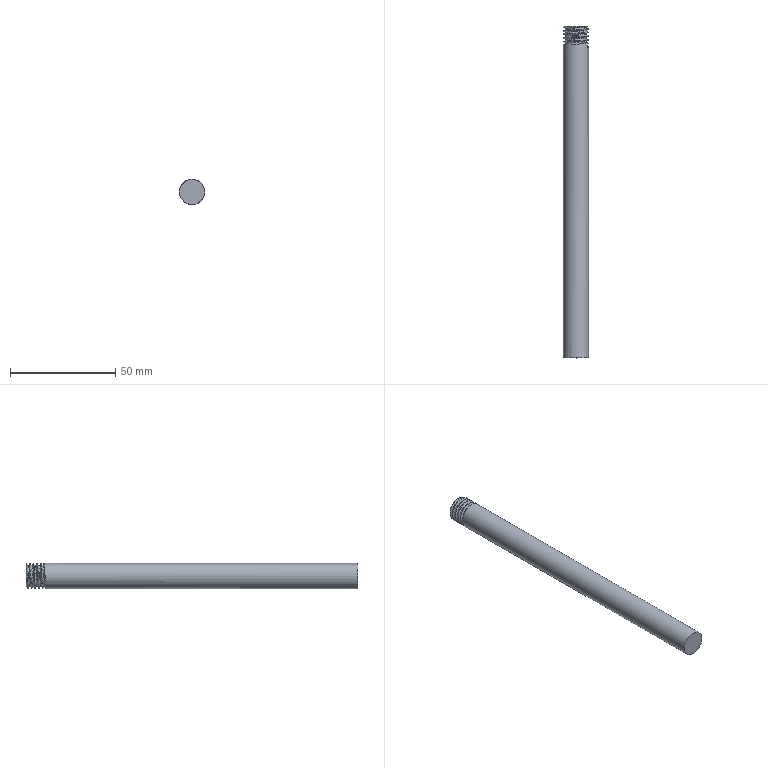Part | STEP file | Tube necking machine_id18_x_t | 1 solid | 13 faces | box 12 x 158 x 12 mm | volume 17697 mm3 | cylinder 7 | plane 3 | spline 2 | cone 1 | commonest cylinder face diameters 12 x6 10.25 x1